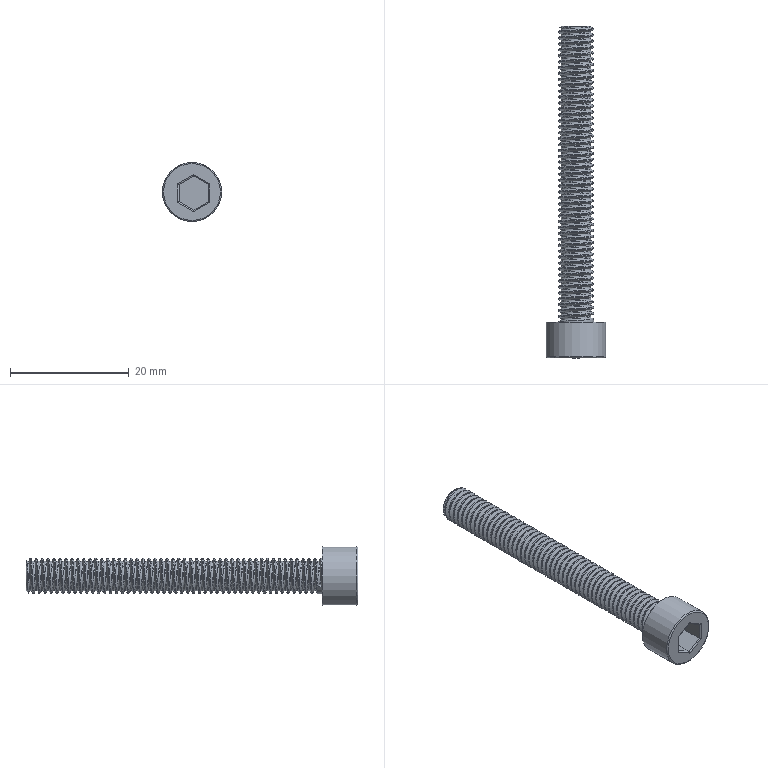Part | STEP file | Tube feed_id990_x_t | 1 solid | 26 faces | box 10 x 56 x 10 mm | volume 1498 mm3 | plane 12 | cylinder 9 | spline 3 | torus 1 | cone 1 | commonest cylinder face diameters 0.4 x6 5 x1 6 x1 10 x1